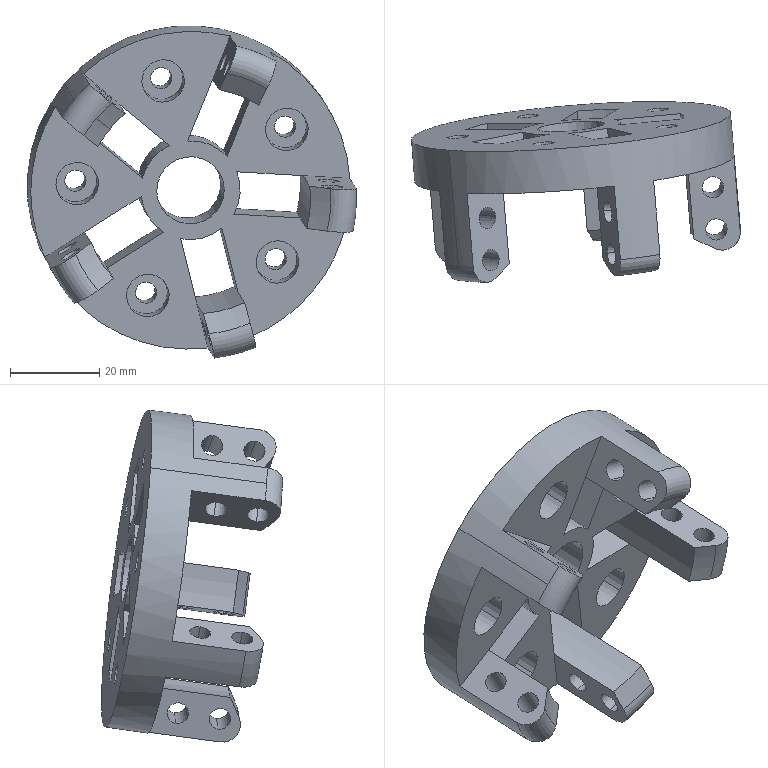Part | SolidWorks | features SplitBody 1 | 1 solid | 93 faces | box 73.96 x 40.675 x 74.65 mm | volume 36556 mm3 | cylinder 55 | plane 27 | cone 6 | torus 5 | commonest cylinder face diameters 4.8 x30 9.6 x10 22.4 x6 51.2 x5 15.2 x2 72 x2